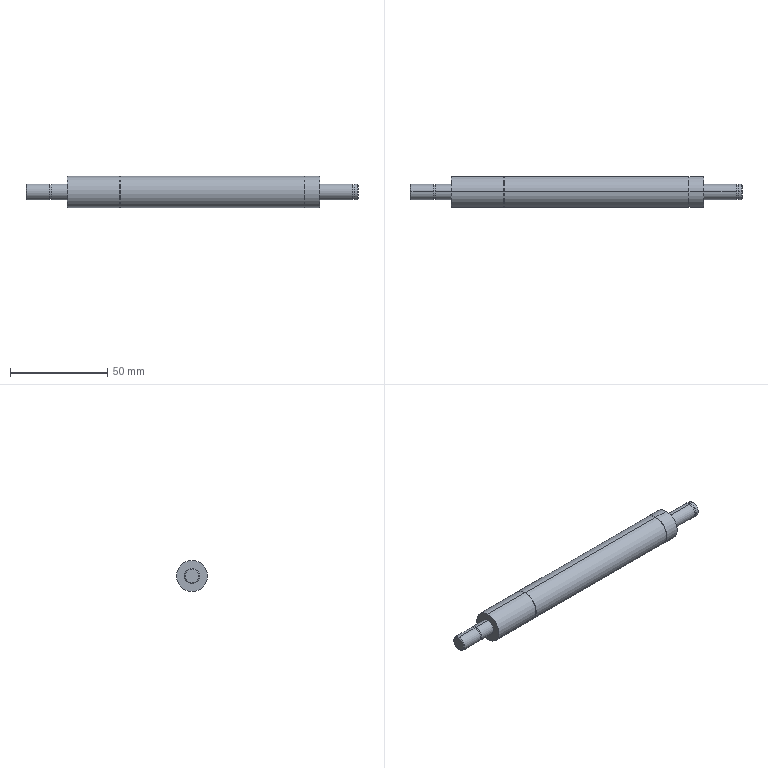Part | SolidWorks | features Chamfer 1, RevCut 1, Revolution 1 | 1 solid | 38 faces | box 171 x 16 x 16 mm | volume 28140 mm3 | cylinder 22 | plane 12 | cone 4 | commonest cylinder face diameters 8 x8 16 x6 7.6 x4 12.8 x4
STEP:
#1=CARTESIAN_POINT('',(171.,0.,-3.5));
#2=VERTEX_POINT('',#1);
#3=CARTESIAN_POINT('',(171.,0.,3.5));
#4=VERTEX_POINT('',#3);
#5=CARTESIAN_POINT('',(171.,0.,0.));
#6=DIRECTION('',(1.,0.,0.));
#7=DIRECTION('',(0.,0.,-1.));
#8=AXIS2_PLACEMENT_3D('',#5,#6,#7);
#9=CIRCLE('',#8,3.5);
#10=EDGE_CURVE('',#2,#4,#9,.T.);
#11=ORIENTED_EDGE('',*,*,#10,.F.);
#12=CARTESIAN_POINT('',(170.5,0.,-4.));
#13=VERTEX_POINT('',#12);
#14=CARTESIAN_POINT('',(170.5,0.,-4.));
#15=DIRECTION('',(-0.7071,0.,-0.7071));
#16=VECTOR('',#15,1000.);
#17=LINE('',#14,#16);
#18=EDGE_CURVE('',#2,#13,#17,.T.);
#19=ORIENTED_EDGE('',*,*,#18,.T.);
#20=CARTESIAN_POINT('',(170.5,0.,4.));
#21=VERTEX_POINT('',#20);
#22=CARTESIAN_POINT('',(170.5,0.,0.));
#23=DIRECTION('',(-1.,0.,0.));
#24=DIRECTION('',(0.,0.,-1.));
#25=AXIS2_PLACEMENT_3D('',#22,#23,#24);
#26=CIRCLE('',#25,4.);
#27=EDGE_CURVE('',#21,#13,#26,.T.);
#28=ORIENTED_EDGE('',*,*,#27,.F.);
#29=CARTESIAN_POINT('',(170.5,0.,4.));
#30=DIRECTION('',(-0.7071,0.,0.7071));
#31=VECTOR('',#30,1000.);
#32=LINE('',#29,#31);
#33=EDGE_CURVE('',#4,#21,#32,.T.);
#34=ORIENTED_EDGE('',*,*,#33,.F.);
#35=EDGE_LOOP('',(#11,#19,#28,#34));
#36=FACE_OUTER_BOUND('',#35,.T.);
#37=CARTESIAN_POINT('',(170.5,0.,0.));
#38=DIRECTION('',(-1.,0.,0.));
#39=DIRECTION('',(0.,0.,1.));
#40=AXIS2_PLACEMENT_3D('',#37,#38,#39);
#41=CONICAL_SURFACE('',#40,4.,0.7854);
#42=ADVANCED_FACE('',(#36),#41,.T.);
#43=CARTESIAN_POINT('',(0.,0.,3.5));
#44=VERTEX_POINT('',#43);
#45=CARTESIAN_POINT('',(0.,0.,-3.5));
#46=VERTEX_POINT('',#45);
#47=CARTESIAN_POINT('',(0.,0.,0.));
#48=DIRECTION('',(-1.,0.,0.));
#49=DIRECTION('',(0.,0.,1.));
#50=AXIS2_PLACEMENT_3D('',#47,#48,#49);
#51=CIRCLE('',#50,3.5);
#52=EDGE_CURVE('',#44,#46,#51,.T.);
#53=ORIENTED_EDGE('',*,*,#52,.F.);
#54=CARTESIAN_POINT('',(0.5,0.,4.));
#55=VERTEX_POINT('',#54);
#56=CARTESIAN_POINT('',(0.,0.,3.5));
#57=DIRECTION('',(0.7071,0.,0.7071));
#58=VECTOR('',#57,1000.);
#59=LINE('',#56,#58);
#60=EDGE_CURVE('',#44,#55,#59,.T.);
#61=ORIENTED_EDGE('',*,*,#60,.T.);
#62=CARTESIAN_POINT('',(0.5,0.,-4.));
#63=VERTEX_POINT('',#62);
#64=CARTESIAN_POINT('',(0.5,0.,0.));
#65=DIRECTION('',(1.,0.,0.));
#66=DIRECTION('',(0.,0.,1.));
#67=AXIS2_PLACEMENT_3D('',#64,#65,#66);
#68=CIRCLE('',#67,4.);
#69=EDGE_CURVE('',#63,#55,#68,.T.);
#70=ORIENTED_EDGE('',*,*,#69,.F.);
#71=CARTESIAN_POINT('',(0.,0.,-3.5));
#72=DIRECTION('',(0.7071,0.,-0.7071));
#73=VECTOR('',#72,1000.);
#74=LINE('',#71,#73);
#75=EDGE_CURVE('',#46,#63,#74,.T.);
#76=ORIENTED_EDGE('',*,*,#75,.F.);
#77=EDGE_LOOP('',(#53,#61,#70,#76));
#78=FACE_OUTER_BOUND('',#77,.T.);
#79=CARTESIAN_POINT('',(0.,0.,0.));
#80=DIRECTION('',(1.,0.,0.));
#81=DIRECTION('',(0.,0.,-1.));
#82=AXIS2_PLACEMENT_3D('',#79,#80,#81);
#83=CONICAL_SURFACE('',#82,3.5,0.7854);
#84=ADVANCED_FACE('',(#78),#83,.T.);
#85=CARTESIAN_POINT('',(12.,0.,4.));
#86=VERTEX_POINT('',#85);
#87=CARTESIAN_POINT('',(12.,0.,-4.));
#88=VERTEX_POINT('',#87);
#89=CARTESIAN_POINT('',(12.,0.,0.));
#90=DIRECTION('',(-1.,0.,0.));
#91=DIRECTION('',(0.,0.,1.));
#92=AXIS2_PLACEMENT_3D('',#89,#90,#91);
#93=CIRCLE('',#92,4.);
#94=EDGE_CURVE('',#86,#88,#93,.T.);
#95=ORIENTED_EDGE('',*,*,#94,.T.);
#96=CARTESIAN_POINT('',(-12.257,0.,-4.));
#97=DIRECTION('',(-1.,0.,0.));
#98=VECTOR('',#97,1000.);
#99=LINE('',#96,#98);
#100=EDGE_CURVE('',#88,#63,#99,.T.);
#101=ORIENTED_EDGE('',*,*,#100,.T.);
#102=ORIENTED_EDGE('',*,*,#69,.T.);
#103=CARTESIAN_POINT('',(-12.257,0.,4.));
#104=DIRECTION('',(-1.,0.,0.));
#105=VECTOR('',#104,1000.);
#106=LINE('',#103,#105);
#107=EDGE_CURVE('',#86,#55,#106,.T.);
#108=ORIENTED_EDGE('',*,*,#107,.F.);
#109=EDGE_LOOP('',(#95,#101,#102,#108));
#110=FACE_OUTER_BOUND('',#109,.T.);
#111=CARTESIAN_POINT('',(-12.257,0.,0.));
#112=DIRECTION('',(-1.,0.,0.));
#113=DIRECTION('',(0.,0.,1.));
#114=AXIS2_PLACEMENT_3D('',#111,#112,#113);
#115=CYLINDRICAL_SURFACE('',#114,4.);
#116=ADVANCED_FACE('',(#110),#115,.T.);
#117=CARTESIAN_POINT('',(12.9,0.,3.8));
#118=VERTEX_POINT('',#117);
#119=CARTESIAN_POINT('',(12.9,0.,-3.8));
#120=VERTEX_POINT('',#119);
#121=CARTESIAN_POINT('',(12.9,0.,0.));
#122=DIRECTION('',(-1.,0.,0.));
#123=DIRECTION('',(0.,0.,1.));
#124=AXIS2_PLACEMENT_3D('',#121,#122,#123);
#125=CIRCLE('',#124,3.8);
#126=EDGE_CURVE('',#118,#120,#125,.T.);
#127=ORIENTED_EDGE('',*,*,#126,.T.);
#128=CARTESIAN_POINT('',(12.,0.,-3.8));
#129=VERTEX_POINT('',#128);
#130=CARTESIAN_POINT('',(-6.355,0.,-3.8));
#131=DIRECTION('',(-1.,0.,0.));
#132=VECTOR('',#131,1000.);
#133=LINE('',#130,#132);
#134=EDGE_CURVE('',#120,#129,#133,.T.);
#135=ORIENTED_EDGE('',*,*,#134,.T.);
#136=CARTESIAN_POINT('',(12.,0.,3.8));
#137=VERTEX_POINT('',#136);
#138=CARTESIAN_POINT('',(12.,0.,0.));
#139=DIRECTION('',(-1.,0.,0.));
#140=DIRECTION('',(0.,0.,1.));
#141=AXIS2_PLACEMENT_3D('',#138,#139,#140);
#142=CIRCLE('',#141,3.8);
#143=EDGE_CURVE('',#137,#129,#142,.T.);
#144=ORIENTED_EDGE('',*,*,#143,.F.);
#145=CARTESIAN_POINT('',(-6.355,0.,3.8));
#146=DIRECTION('',(-1.,0.,0.));
#147=VECTOR('',#146,1000.);
#148=LINE('',#145,#147);
#149=EDGE_CURVE('',#118,#137,#148,.T.);
#150=ORIENTED_EDGE('',*,*,#149,.F.);
#151=EDGE_LOOP('',(#127,#135,#144,#150));
#152=FACE_OUTER_BOUND('',#151,.T.);
#153=CARTESIAN_POINT('',(-6.355,0.,0.));
#154=DIRECTION('',(-1.,0.,0.));
#155=DIRECTION('',(0.,0.,1.));
#156=AXIS2_PLACEMENT_3D('',#153,#154,#155);
#157=CYLINDRICAL_SURFACE('',#156,3.8);
#158=ADVANCED_FACE('',(#152),#157,.T.);
#159=ORIENTED_EDGE('',*,*,#27,.T.);
#160=CARTESIAN_POINT('',(169.,0.,-4.));
#161=VERTEX_POINT('',#160);
#162=CARTESIAN_POINT('',(-12.257,0.,-4.));
#163=DIRECTION('',(-1.,0.,0.));
#164=VECTOR('',#163,1000.);
#165=LINE('',#162,#164);
#166=EDGE_CURVE('',#13,#161,#165,.T.);
#167=ORIENTED_EDGE('',*,*,#166,.T.);
#168=CARTESIAN_POINT('',(169.,0.,4.));
#169=VERTEX_POINT('',#168);
#170=CARTESIAN_POINT('',(169.,0.,0.));
#171=DIRECTION('',(-1.,0.,0.));
#172=DIRECTION('',(0.,0.,1.));
#173=AXIS2_PLACEMENT_3D('',#170,#171,#172);
#174=CIRCLE('',#173,4.);
#175=EDGE_CURVE('',#169,#161,#174,.T.);
#176=ORIENTED_EDGE('',*,*,#175,.F.);
#177=CARTESIAN_POINT('',(-12.257,0.,4.));
#178=DIRECTION('',(-1.,0.,0.));
#179=VECTOR('',#178,1000.);
#180=LINE('',#177,#179);
#181=EDGE_CURVE('',#21,#169,#180,.T.);
#182=ORIENTED_EDGE('',*,*,#181,.F.);
#183=EDGE_LOOP('',(#159,#167,#176,#182));
#184=FACE_OUTER_BOUND('',#183,.T.);
#185=CARTESIAN_POINT('',(-12.257,0.,0.));
#186=DIRECTION('',(-1.,0.,0.));
#187=DIRECTION('',(0.,0.,1.));
#188=AXIS2_PLACEMENT_3D('',#185,#186,#187);
#189=CYLINDRICAL_SURFACE('',#188,4.);
#190=ADVANCED_FACE('',(#184),#189,.T.);
#191=CARTESIAN_POINT('',(169.,0.,3.8));
#192=VERTEX_POINT('',#191);
#193=CARTESIAN_POINT('',(169.,0.,-3.8));
#194=VERTEX_POINT('',#193);
#195=CARTESIAN_POINT('',(169.,0.,0.));
#196=DIRECTION('',(-1.,0.,0.));
#197=DIRECTION('',(0.,0.,1.));
#198=AXIS2_PLACEMENT_3D('',#195,#196,#197);
#199=CIRCLE('',#198,3.8);
#200=EDGE_CURVE('',#192,#194,#199,.T.);
#201=ORIENTED_EDGE('',*,*,#200,.T.);
#202=CARTESIAN_POINT('',(168.1,0.,-3.8));
#203=VERTEX_POINT('',#202);
#204=CARTESIAN_POINT('',(-6.355,0.,-3.8));
#205=DIRECTION('',(-1.,0.,0.));
#206=VECTOR('',#205,1000.);
#207=LINE('',#204,#206);
#208=EDGE_CURVE('',#194,#203,#207,.T.);
#209=ORIENTED_EDGE('',*,*,#208,.T.);
#210=CARTESIAN_POINT('',(168.1,0.,3.8));
#211=VERTEX_POINT('',#210);
#212=CARTESIAN_POINT('',(168.1,0.,0.));
#213=DIRECTION('',(-1.,0.,0.));
#214=DIRECTION('',(0.,0.,1.));
#215=AXIS2_PLACEMENT_3D('',#212,#213,#214);
#216=CIRCLE('',#215,3.8);
#217=EDGE_CURVE('',#211,#203,#216,.T.);
#218=ORIENTED_EDGE('',*,*,#217,.F.);
#219=CARTESIAN_POINT('',(-6.355,0.,3.8));
#220=DIRECTION('',(-1.,0.,0.));
#221=VECTOR('',#220,1000.);
#222=LINE('',#219,#221);
#223=EDGE_CURVE('',#192,#211,#222,.T.);
#224=ORIENTED_EDGE('',*,*,#223,.F.);
#225=EDGE_LOOP('',(#201,#209,#218,#224));
#226=FACE_OUTER_BOUND('',#225,.T.);
#227=CARTESIAN_POINT('',(-6.355,0.,0.));
#228=DIRECTION('',(-1.,0.,0.));
#229=DIRECTION('',(0.,0.,1.));
#230=AXIS2_PLACEMENT_3D('',#227,#228,#229);
#231=CYLINDRICAL_SURFACE('',#230,3.8);
#232=ADVANCED_FACE('',(#226),#231,.T.);
#233=CARTESIAN_POINT('',(151.2,0.,8.));
#234=VERTEX_POINT('',#233);
#235=CARTESIAN_POINT('',(151.2,0.,-8.));
#236=VERTEX_POINT('',#235);
#237=CARTESIAN_POINT('',(151.2,0.,0.));
#238=DIRECTION('',(-1.,0.,0.));
#239=DIRECTION('',(0.,0.,1.));
#240=AXIS2_PLACEMENT_3D('',#237,#238,#239);
#241=CIRCLE('',#240,8.);
#242=EDGE_CURVE('',#234,#236,#241,.T.);
#243=ORIENTED_EDGE('',*,*,#242,.T.);
#244=CARTESIAN_POINT('',(143.7,0.,-8.));
#245=VERTEX_POINT('',#244);
#246=CARTESIAN_POINT('',(-12.257,0.,-8.));
#247=DIRECTION('',(-1.,0.,0.));
#248=VECTOR('',#247,1000.);
#249=LINE('',#246,#248);
#250=EDGE_CURVE('',#236,#245,#249,.T.);
#251=ORIENTED_EDGE('',*,*,#250,.T.);
#252=CARTESIAN_POINT('',(143.7,0.,8.));
#253=VERTEX_POINT('',#252);
#254=CARTESIAN_POINT('',(143.7,0.,0.));
#255=DIRECTION('',(-1.,0.,0.));
#256=DIRECTION('',(0.,0.,1.));
#257=AXIS2_PLACEMENT_3D('',#254,#255,#256);
#258=CIRCLE('',#257,8.);
#259=EDGE_CURVE('',#253,#245,#258,.T.);
#260=ORIENTED_EDGE('',*,*,#259,.F.);
#261=CARTESIAN_POINT('',(-12.257,0.,8.));
#262=DIRECTION('',(-1.,0.,0.));
#263=VECTOR('',#262,1000.);
#264=LINE('',#261,#263);
#265=EDGE_CURVE('',#234,#253,#264,.T.);
#266=ORIENTED_EDGE('',*,*,#265,.F.);
#267=EDGE_LOOP('',(#243,#251,#260,#266));
#268=FACE_OUTER_BOUND('',#267,.T.);
#269=CARTESIAN_POINT('',(-12.257,0.,0.));
#270=DIRECTION('',(-1.,0.,0.));
#271=DIRECTION('',(0.,0.,1.));
#272=AXIS2_PLACEMENT_3D('',#269,#270,#271);
#273=CYLINDRICAL_SURFACE('',#272,8.);
#274=ADVANCED_FACE('',(#268),#273,.T.);
#275=CARTESIAN_POINT('',(143.7,0.,6.4));
#276=VERTEX_POINT('',#275);
#277=CARTESIAN_POINT('',(143.7,0.,-6.4));
#278=VERTEX_POINT('',#277);
#279=CARTESIAN_POINT('',(143.7,0.,0.));
#280=DIRECTION('',(-1.,0.,0.));
#281=DIRECTION('',(0.,0.,1.));
#282=AXIS2_PLACEMENT_3D('',#279,#280,#281);
#283=CIRCLE('',#282,6.4);
#284=EDGE_CURVE('',#276,#278,#283,.T.);
#285=ORIENTED_EDGE('',*,*,#284,.T.);
#286=CARTESIAN_POINT('',(143.5,0.,-6.4));
#287=VERTEX_POINT('',#286);
#288=CARTESIAN_POINT('',(-6.355,0.,-6.4));
#289=DIRECTION('',(-1.,0.,0.));
#290=VECTOR('',#289,1000.);
#291=LINE('',#288,#290);
#292=EDGE_CURVE('',#278,#287,#291,.T.);
#293=ORIENTED_EDGE('',*,*,#292,.T.);
#294=CARTESIAN_POINT('',(143.5,0.,6.4));
#295=VERTEX_POINT('',#294);
#296=CARTESIAN_POINT('',(143.5,0.,0.));
#297=DIRECTION('',(-1.,0.,0.));
#298=DIRECTION('',(0.,0.,1.));
#299=AXIS2_PLACEMENT_3D('',#296,#297,#298);
#300=CIRCLE('',#299,6.4);
#301=EDGE_CURVE('',#295,#287,#300,.T.);
#302=ORIENTED_EDGE('',*,*,#301,.F.);
#303=CARTESIAN_POINT('',(-6.355,0.,6.4));
#304=DIRECTION('',(-1.,0.,0.));
#305=VECTOR('',#304,1000.);
#306=LINE('',#303,#305);
#307=EDGE_CURVE('',#276,#295,#306,.T.);
#308=ORIENTED_EDGE('',*,*,#307,.F.);
#309=EDGE_LOOP('',(#285,#293,#302,#308));
#310=FACE_OUTER_BOUND('',#309,.T.);
#311=CARTESIAN_POINT('',(-6.355,0.,0.));
#312=DIRECTION('',(-1.,0.,0.));
#313=DIRECTION('',(0.,0.,1.));
#314=AXIS2_PLACEMENT_3D('',#311,#312,#313);
#315=CYLINDRICAL_SURFACE('',#314,6.4);
#316=ADVANCED_FACE('',(#310),#315,.T.);
#317=CARTESIAN_POINT('',(48.5,0.,6.4));
#318=VERTEX_POINT('',#317);
#319=CARTESIAN_POINT('',(48.5,0.,-6.4));
#320=VERTEX_POINT('',#319);
#321=CARTESIAN_POINT('',(48.5,0.,0.));
#322=DIRECTION('',(-1.,0.,0.));
#323=DIRECTION('',(0.,0.,1.));
#324=AXIS2_PLACEMENT_3D('',#321,#322,#323);
#325=CIRCLE('',#324,6.4);
#326=EDGE_CURVE('',#318,#320,#325,.T.);
#327=ORIENTED_EDGE('',*,*,#326,.T.);
#328=CARTESIAN_POINT('',(48.3,0.,-6.4));
#329=VERTEX_POINT('',#328);
#330=CARTESIAN_POINT('',(-6.355,0.,-6.4));
#331=DIRECTION('',(-1.,0.,0.));
#332=VECTOR('',#331,1000.);
#333=LINE('',#330,#332);
#334=EDGE_CURVE('',#320,#329,#333,.T.);
#335=ORIENTED_EDGE('',*,*,#334,.T.);
#336=CARTESIAN_POINT('',(48.3,0.,6.4));
#337=VERTEX_POINT('',#336);
#338=CARTESIAN_POINT('',(48.3,0.,0.));
#339=DIRECTION('',(-1.,0.,0.));
#340=DIRECTION('',(0.,0.,1.));
#341=AXIS2_PLACEMENT_3D('',#338,#339,#340);
#342=CIRCLE('',#341,6.4);
#343=EDGE_CURVE('',#337,#329,#342,.T.);
#344=ORIENTED_EDGE('',*,*,#343,.F.);
#345=CARTESIAN_POINT('',(-6.355,0.,6.4));
#346=DIRECTION('',(-1.,0.,0.));
#347=VECTOR('',#346,1000.);
#348=LINE('',#345,#347);
#349=EDGE_CURVE('',#318,#337,#348,.T.);
#350=ORIENTED_EDGE('',*,*,#349,.F.);
#351=EDGE_LOOP('',(#327,#335,#344,#350));
#352=FACE_OUTER_BOUND('',#351,.T.);
#353=CARTESIAN_POINT('',(-6.355,0.,0.));
#354=DIRECTION('',(-1.,0.,0.));
#355=DIRECTION('',(0.,0.,1.));
#356=AXIS2_PLACEMENT_3D('',#353,#354,#355);
#357=CYLINDRICAL_SURFACE('',#356,6.4);
#358=ADVANCED_FACE('',(#352),#357,.T.);
#359=CARTESIAN_POINT('',(21.3,0.,4.));
#360=VERTEX_POINT('',#359);
#361=CARTESIAN_POINT('',(21.3,0.,-4.));
#362=VERTEX_POINT('',#361);
#363=CARTESIAN_POINT('',(21.3,0.,0.));
#364=DIRECTION('',(-1.,0.,0.));
#365=DIRECTION('',(0.,0.,1.));
#366=AXIS2_PLACEMENT_3D('',#363,#364,#365);
#367=CIRCLE('',#366,4.);
#368=EDGE_CURVE('',#360,#362,#367,.T.);
#369=ORIENTED_EDGE('',*,*,#368,.T.);
#370=CARTESIAN_POINT('',(12.9,0.,-4.));
#371=VERTEX_POINT('',#370);
#372=CARTESIAN_POINT('',(-12.257,0.,-4.));
#373=DIRECTION('',(-1.,0.,0.));
#374=VECTOR('',#373,1000.);
#375=LINE('',#372,#374);
#376=EDGE_CURVE('',#362,#371,#375,.T.);
#377=ORIENTED_EDGE('',*,*,#376,.T.);
#378=CARTESIAN_POINT('',(12.9,0.,4.));
#379=VERTEX_POINT('',#378);
#380=CARTESIAN_POINT('',(12.9,0.,0.));
#381=DIRECTION('',(-1.,0.,0.));
#382=DIRECTION('',(0.,0.,1.));
#383=AXIS2_PLACEMENT_3D('',#380,#381,#382);
#384=CIRCLE('',#383,4.);
#385=EDGE_CURVE('',#379,#371,#384,.T.);
#386=ORIENTED_EDGE('',*,*,#385,.F.);
#387=CARTESIAN_POINT('',(-12.257,0.,4.));
#388=DIRECTION('',(-1.,0.,0.));
#389=VECTOR('',#388,1000.);
#390=LINE('',#387,#389);
#391=EDGE_CURVE('',#360,#379,#390,.T.);
#392=ORIENTED_EDGE('',*,*,#391,.F.);
#393=EDGE_LOOP('',(#369,#377,#386,#392));
#394=FACE_OUTER_BOUND('',#393,.T.);
#395=CARTESIAN_POINT('',(-12.257,0.,0.));
#396=DIRECTION('',(-1.,0.,0.));
#397=DIRECTION('',(0.,0.,1.));
#398=AXIS2_PLACEMENT_3D('',#395,#396,#397);
#399=CYLINDRICAL_SURFACE('',#398,4.);
#400=ADVANCED_FACE('',(#394),#399,.T.);
#401=CARTESIAN_POINT('',(48.3,0.,8.));
#402=VERTEX_POINT('',#401);
#403=CARTESIAN_POINT('',(48.3,0.,-8.));
#404=VERTEX_POINT('',#403);
#405=CARTESIAN_POINT('',(48.3,0.,0.));
#406=DIRECTION('',(-1.,0.,0.));
#407=DIRECTION('',(0.,0.,1.));
#408=AXIS2_PLACEMENT_3D('',#405,#406,#407);
#409=CIRCLE('',#408,8.);
#410=EDGE_CURVE('',#402,#404,#409,.T.);
#411=ORIENTED_EDGE('',*,*,#410,.T.);
#412=CARTESIAN_POINT('',(21.3,0.,-8.));
#413=VERTEX_POINT('',#412);
#414=CARTESIAN_POINT('',(-12.257,0.,-8.));
#415=DIRECTION('',(-1.,0.,0.));
#416=VECTOR('',#415,1000.);
#417=LINE('',#414,#416);
#418=EDGE_CURVE('',#404,#413,#417,.T.);
#419=ORIENTED_EDGE('',*,*,#418,.T.);
#420=CARTESIAN_POINT('',(21.3,0.,8.));
#421=VERTEX_POINT('',#420);
#422=CARTESIAN_POINT('',(21.3,0.,0.));
#423=DIRECTION('',(-1.,0.,0.));
#424=DIRECTION('',(0.,0.,1.));
#425=AXIS2_PLACEMENT_3D('',#422,#423,#424);
#426=CIRCLE('',#425,8.);
#427=EDGE_CURVE('',#421,#413,#426,.T.);
#428=ORIENTED_EDGE('',*,*,#427,.F.);
#429=CARTESIAN_POINT('',(-12.257,0.,8.));
#430=DIRECTION('',(-1.,0.,0.));
#431=VECTOR('',#430,1000.);
#432=LINE('',#429,#431);
#433=EDGE_CURVE('',#402,#421,#432,.T.);
#434=ORIENTED_EDGE('',*,*,#433,.F.);
#435=EDGE_LOOP('',(#411,#419,#428,#434));
#436=FACE_OUTER_BOUND('',#435,.T.);
#437=CARTESIAN_POINT('',(-12.257,0.,0.));
#438=DIRECTION('',(-1.,0.,0.));
#439=DIRECTION('',(0.,0.,1.));
#440=AXIS2_PLACEMENT_3D('',#437,#438,#439);
#441=CYLINDRICAL_SURFACE('',#440,8.);
#442=ADVANCED_FACE('',(#436),#441,.T.);
#443=CARTESIAN_POINT('',(143.5,0.,8.));
#444=VERTEX_POINT('',#443);
#445=CARTESIAN_POINT('',(143.5,0.,-8.));
#446=VERTEX_POINT('',#445);
#447=CARTESIAN_POINT('',(143.5,0.,0.));
#448=DIRECTION('',(-1.,0.,0.));
#449=DIRECTION('',(0.,0.,1.));
#450=AXIS2_PLACEMENT_3D('',#447,#448,#449);
#451=CIRCLE('',#450,8.);
#452=EDGE_CURVE('',#444,#446,#451,.T.);
#453=ORIENTED_EDGE('',*,*,#452,.T.);
#454=CARTESIAN_POINT('',(48.5,0.,-8.));
#455=VERTEX_POINT('',#454);
#456=CARTESIAN_POINT('',(-12.257,0.,-8.));
#457=DIRECTION('',(-1.,0.,0.));
#458=VECTOR('',#457,1000.);
#459=LINE('',#456,#458);
#460=EDGE_CURVE('',#446,#455,#459,.T.);
#461=ORIENTED_EDGE('',*,*,#460,.T.);
#462=CARTESIAN_POINT('',(48.5,0.,8.));
#463=VERTEX_POINT('',#462);
#464=CARTESIAN_POINT('',(48.5,0.,0.));
#465=DIRECTION('',(-1.,0.,0.));
#466=DIRECTION('',(0.,0.,1.));
#467=AXIS2_PLACEMENT_3D('',#464,#465,#466);
#468=CIRCLE('',#467,8.);
#469=EDGE_CURVE('',#463,#455,#468,.T.);
#470=ORIENTED_EDGE('',*,*,#469,.F.);
#471=CARTESIAN_POINT('',(-12.257,0.,8.));
#472=DIRECTION('',(-1.,0.,0.));
#473=VECTOR('',#472,1000.);
#474=LINE('',#471,#473);
#475=EDGE_CURVE('',#444,#463,#474,.T.);
#476=ORIENTED_EDGE('',*,*,#475,.F.);
#477=EDGE_LOOP('',(#453,#461,#470,#476));
#478=FACE_OUTER_BOUND('',#477,.T.);
#479=CARTESIAN_POINT('',(-12.257,0.,0.));
#480=DIRECTION('',(-1.,0.,0.));
#481=DIRECTION('',(0.,0.,1.));
#482=AXIS2_PLACEMENT_3D('',#479,#480,#481);
#483=CYLINDRICAL_SURFACE('',#482,8.);
#484=ADVANCED_FACE('',(#478),#483,.T.);
#485=CARTESIAN_POINT('',(168.1,0.,4.));
#486=VERTEX_POINT('',#485);
#487=CARTESIAN_POINT('',(168.1,0.,-4.));
#488=VERTEX_POINT('',#487);
#489=CARTESIAN_POINT('',(168.1,0.,0.));
#490=DIRECTION('',(-1.,0.,0.));
#491=DIRECTION('',(0.,0.,1.));
#492=AXIS2_PLACEMENT_3D('',#489,#490,#491);
#493=CIRCLE('',#492,4.);
#494=EDGE_CURVE('',#486,#488,#493,.T.);
#495=ORIENTED_EDGE('',*,*,#494,.T.);
#496=CARTESIAN_POINT('',(151.2,0.,-4.));
#497=VERTEX_POINT('',#496);
#498=CARTESIAN_POINT('',(-12.257,0.,-4.));
#499=DIRECTION('',(-1.,0.,0.));
#500=VECTOR('',#499,1000.);
#501=LINE('',#498,#500);
#502=EDGE_CURVE('',#488,#497,#501,.T.);
#503=ORIENTED_EDGE('',*,*,#502,.T.);
#504=CARTESIAN_POINT('',(151.2,0.,4.));
#505=VERTEX_POINT('',#504);
#506=CARTESIAN_POINT('',(151.2,0.,0.));
#507=DIRECTION('',(-1.,0.,0.));
#508=DIRECTION('',(0.,0.,1.));
#509=AXIS2_PLACEMENT_3D('',#506,#507,#508);
#510=CIRCLE('',#509,4.);
#511=EDGE_CURVE('',#505,#497,#510,.T.);
#512=ORIENTED_EDGE('',*,*,#511,.F.);
#513=CARTESIAN_POINT('',(-12.257,0.,4.));
#514=DIRECTION('',(-1.,0.,0.));
#515=VECTOR('',#514,1000.);
#516=LINE('',#513,#515);
#517=EDGE_CURVE('',#486,#505,#516,.T.);
#518=ORIENTED_EDGE('',*,*,#517,.F.);
#519=EDGE_LOOP('',(#495,#503,#512,#518));
#520=FACE_OUTER_BOUND('',#519,.T.);
#521=CARTESIAN_POINT('',(-12.257,0.,0.));
#522=DIRECTION('',(-1.,0.,0.));
#523=DIRECTION('',(0.,0.,1.));
#524=AXIS2_PLACEMENT_3D('',#521,#522,#523);
#525=CYLINDRICAL_SURFACE('',#524,4.);
#526=ADVANCED_FACE('',(#520),#525,.T.);
#527=ORIENTED_EDGE('',*,*,#502,.F.);
#528=CARTESIAN_POINT('',(168.1,0.,0.));
#529=DIRECTION('',(-1.,0.,0.));
#530=DIRECTION('',(0.,0.,1.));
#531=AXIS2_PLACEMENT_3D('',#528,#529,#530);
#532=CIRCLE('',#531,4.);
#533=EDGE_CURVE('',#488,#486,#532,.T.);
#534=ORIENTED_EDGE('',*,*,#533,.T.);
#535=ORIENTED_EDGE('',*,*,#517,.T.);
#536=CARTESIAN_POINT('',(151.2,0.,0.));
#537=DIRECTION('',(-1.,0.,0.));
#538=DIRECTION('',(0.,0.,1.));
#539=AXIS2_PLACEMENT_3D('',#536,#537,#538);
#540=CIRCLE('',#539,4.);
#541=EDGE_CURVE('',#497,#505,#540,.T.);
#542=ORIENTED_EDGE('',*,*,#541,.F.);
#543=EDGE_LOOP('',(#527,#534,#535,#542));
#544=FACE_OUTER_BOUND('',#543,.T.);
#545=CARTESIAN_POINT('',(-12.257,0.,0.));
#546=DIRECTION('',(-1.,0.,0.));
#547=DIRECTION('',(0.,0.,1.));
#548=AXIS2_PLACEMENT_3D('',#545,#546,#547);
#549=CYLINDRICAL_SURFACE('',#548,4.);
#550=ADVANCED_FACE('',(#544),#549,.T.);
#551=ORIENTED_EDGE('',*,*,#460,.F.);
#552=CARTESIAN_POINT('',(143.5,0.,0.));
#553=DIRECTION('',(-1.,0.,0.));
#554=DIRECTION('',(0.,0.,1.));
#555=AXIS2_PLACEMENT_3D('',#552,#553,#554);
#556=CIRCLE('',#555,8.);
#557=EDGE_CURVE('',#446,#444,#556,.T.);
#558=ORIENTED_EDGE('',*,*,#557,.T.);
#559=ORIENTED_EDGE('',*,*,#475,.T.);
#560=CARTESIAN_POINT('',(48.5,0.,0.));
#561=DIRECTION('',(-1.,0.,0.));
#562=DIRECTION('',(0.,0.,1.));
#563=AXIS2_PLACEMENT_3D('',#560,#561,#562);
#564=CIRCLE('',#563,8.);
#565=EDGE_CURVE('',#455,#463,#564,.T.);
#566=ORIENTED_EDGE('',*,*,#565,.F.);
#567=EDGE_LOOP('',(#551,#558,#559,#566));
#568=FACE_OUTER_BOUND('',#567,.T.);
#569=CARTESIAN_POINT('',(-12.257,0.,0.));
#570=DIRECTION('',(-1.,0.,0.));
#571=DIRECTION('',(0.,0.,1.));
#572=AXIS2_PLACEMENT_3D('',#569,#570,#571);
#573=CYLINDRICAL_SURFACE('',#572,8.);
#574=ADVANCED_FACE('',(#568),#573,.T.);
#575=ORIENTED_EDGE('',*,*,#418,.F.);
#576=CARTESIAN_POINT('',(48.3,0.,0.));
#577=DIRECTION('',(-1.,0.,0.));
#578=DIRECTION('',(0.,0.,1.));
#579=AXIS2_PLACEMENT_3D('',#576,#577,#578);
#580=CIRCLE('',#579,8.);
#581=EDGE_CURVE('',#404,#402,#580,.T.);
#582=ORIENTED_EDGE('',*,*,#581,.T.);
#583=ORIENTED_EDGE('',*,*,#433,.T.);
#584=CARTESIAN_POINT('',(21.3,0.,0.));
#585=DIRECTION('',(-1.,0.,0.));
#586=DIRECTION('',(0.,0.,1.));
#587=AXIS2_PLACEMENT_3D('',#584,#585,#586);
#588=CIRCLE('',#587,8.);
#589=EDGE_CURVE('',#413,#421,#588,.T.);
#590=ORIENTED_EDGE('',*,*,#589,.F.);
#591=EDGE_LOOP('',(#575,#582,#583,#590));
#592=FACE_OUTER_BOUND('',#591,.T.);
#593=CARTESIAN_POINT('',(-12.257,0.,0.));
#594=DIRECTION('',(-1.,0.,0.));
#595=DIRECTION('',(0.,0.,1.));
#596=AXIS2_PLACEMENT_3D('',#593,#594,#595);
#597=CYLINDRICAL_SURFACE('',#596,8.);
#598=ADVANCED_FACE('',(#592),#597,.T.);
#599=ORIENTED_EDGE('',*,*,#376,.F.);
#600=CARTESIAN_POINT('',(21.3,0.,0.));
#601=DIRECTION('',(-1.,0.,0.));
#602=DIRECTION('',(0.,0.,1.));
#603=AXIS2_PLACEMENT_3D('',#600,#601,#602);
#604=CIRCLE('',#603,4.);
#605=EDGE_CURVE('',#362,#360,#604,.T.);
#606=ORIENTED_EDGE('',*,*,#605,.T.);
#607=ORIENTED_EDGE('',*,*,#391,.T.);
#608=CARTESIAN_POINT('',(12.9,0.,0.));
#609=DIRECTION('',(-1.,0.,0.));
#610=DIRECTION('',(0.,0.,1.));
#611=AXIS2_PLACEMENT_3D('',#608,#609,#610);
#612=CIRCLE('',#611,4.);
#613=EDGE_CURVE('',#371,#379,#612,.T.);
#614=ORIENTED_EDGE('',*,*,#613,.F.);
#615=EDGE_LOOP('',(#599,#606,#607,#614));
#616=FACE_OUTER_BOUND('',#615,.T.);
#617=CARTESIAN_POINT('',(-12.257,0.,0.));
#618=DIRECTION('',(-1.,0.,0.));
#619=DIRECTION('',(0.,0.,1.));
#620=AXIS2_PLACEMENT_3D('',#617,#618,#619);
#621=CYLINDRICAL_SURFACE('',#620,4.);
#622=ADVANCED_FACE('',(#616),#621,.T.);
#623=ORIENTED_EDGE('',*,*,#427,.T.);
#624=ORIENTED_EDGE('',*,*,#589,.T.);
#625=EDGE_LOOP('',(#623,#624));
#626=FACE_OUTER_BOUND('',#625,.T.);
#627=ORIENTED_EDGE('',*,*,#368,.F.);
#628=ORIENTED_EDGE('',*,*,#605,.F.);
#629=EDGE_LOOP('',(#627,#628));
#630=FACE_BOUND('',#629,.T.);
#631=CARTESIAN_POINT('',(21.3,0.,-4.));
#632=DIRECTION('',(-1.,0.,0.));
#633=DIRECTION('',(0.,0.,1.));
#634=AXIS2_PLACEMENT_3D('',#631,#632,#633);
#635=PLANE('',#634);
#636=ADVANCED_FACE('',(#626,#630),#635,.T.);
#637=ORIENTED_EDGE('',*,*,#410,.F.);
#638=ORIENTED_EDGE('',*,*,#581,.F.);
#639=EDGE_LOOP('',(#637,#638));
#640=FACE_OUTER_BOUND('',#639,.T.);
#641=ORIENTED_EDGE('',*,*,#343,.T.);
#642=CARTESIAN_POINT('',(48.3,0.,0.));
#643=DIRECTION('',(-1.,0.,0.));
#644=DIRECTION('',(0.,0.,1.));
#645=AXIS2_PLACEMENT_3D('',#642,#643,#644);
#646=CIRCLE('',#645,6.4);
#647=EDGE_CURVE('',#329,#337,#646,.T.);
#648=ORIENTED_EDGE('',*,*,#647,.T.);
#649=EDGE_LOOP('',(#641,#648));
#650=FACE_BOUND('',#649,.T.);
#651=CARTESIAN_POINT('',(48.3,0.,-8.));
#652=DIRECTION('',(-1.,0.,0.));
#653=DIRECTION('',(0.,0.,1.));
#654=AXIS2_PLACEMENT_3D('',#651,#652,#653);
#655=PLANE('',#654);
#656=ADVANCED_FACE('',(#640,#650),#655,.F.);
#657=ORIENTED_EDGE('',*,*,#334,.F.);
#658=CARTESIAN_POINT('',(48.5,0.,0.));
#659=DIRECTION('',(-1.,0.,0.));
#660=DIRECTION('',(0.,0.,1.));
#661=AXIS2_PLACEMENT_3D('',#658,#659,#660);
#662=CIRCLE('',#661,6.4);
#663=EDGE_CURVE('',#320,#318,#662,.T.);
#664=ORIENTED_EDGE('',*,*,#663,.T.);
#665=ORIENTED_EDGE('',*,*,#349,.T.);
#666=ORIENTED_EDGE('',*,*,#647,.F.);
#667=EDGE_LOOP('',(#657,#664,#665,#666));
#668=FACE_OUTER_BOUND('',#667,.T.);
#669=CARTESIAN_POINT('',(-6.355,0.,0.));
#670=DIRECTION('',(-1.,0.,0.));
#671=DIRECTION('',(0.,0.,1.));
#672=AXIS2_PLACEMENT_3D('',#669,#670,#671);
#673=CYLINDRICAL_SURFACE('',#672,6.4);
#674=ADVANCED_FACE('',(#668),#673,.T.);
#675=ORIENTED_EDGE('',*,*,#326,.F.);
#676=ORIENTED_EDGE('',*,*,#663,.F.);
#677=EDGE_LOOP('',(#675,#676));
#678=FACE_BOUND('',#677,.T.);
#679=ORIENTED_EDGE('',*,*,#469,.T.);
#680=ORIENTED_EDGE('',*,*,#565,.T.);
#681=EDGE_LOOP('',(#679,#680));
#682=FACE_OUTER_BOUND('',#681,.T.);
#683=CARTESIAN_POINT('',(48.5,0.,-8.));
#684=DIRECTION('',(1.,0.,0.));
#685=DIRECTION('',(0.,0.,-1.));
#686=AXIS2_PLACEMENT_3D('',#683,#684,#685);
#687=PLANE('',#686);
#688=ADVANCED_FACE('',(#678,#682),#687,.F.);
#689=ORIENTED_EDGE('',*,*,#452,.F.);
#690=ORIENTED_EDGE('',*,*,#557,.F.);
#691=EDGE_LOOP('',(#689,#690));
#692=FACE_OUTER_BOUND('',#691,.T.);
#693=ORIENTED_EDGE('',*,*,#301,.T.);
#694=CARTESIAN_POINT('',(143.5,0.,0.));
#695=DIRECTION('',(-1.,0.,0.));
#696=DIRECTION('',(0.,0.,1.));
#697=AXIS2_PLACEMENT_3D('',#694,#695,#696);
#698=CIRCLE('',#697,6.4);
#699=EDGE_CURVE('',#287,#295,#698,.T.);
#700=ORIENTED_EDGE('',*,*,#699,.T.);
#701=EDGE_LOOP('',(#693,#700));
#702=FACE_BOUND('',#701,.T.);
#703=CARTESIAN_POINT('',(143.5,0.,-8.));
#704=DIRECTION('',(-1.,0.,0.));
#705=DIRECTION('',(0.,0.,1.));
#706=AXIS2_PLACEMENT_3D('',#703,#704,#705);
#707=PLANE('',#706);
#708=ADVANCED_FACE('',(#692,#702),#707,.F.);
#709=ORIENTED_EDGE('',*,*,#292,.F.);
#710=CARTESIAN_POINT('',(143.7,0.,0.));
#711=DIRECTION('',(-1.,0.,0.));
#712=DIRECTION('',(0.,0.,1.));
#713=AXIS2_PLACEMENT_3D('',#710,#711,#712);
#714=CIRCLE('',#713,6.4);
#715=EDGE_CURVE('',#278,#276,#714,.T.);
#716=ORIENTED_EDGE('',*,*,#715,.T.);
#717=ORIENTED_EDGE('',*,*,#307,.T.);
#718=ORIENTED_EDGE('',*,*,#699,.F.);
#719=EDGE_LOOP('',(#709,#716,#717,#718));
#720=FACE_OUTER_BOUND('',#719,.T.);
#721=CARTESIAN_POINT('',(-6.355,0.,0.));
#722=DIRECTION('',(-1.,0.,0.));
#723=DIRECTION('',(0.,0.,1.));
#724=AXIS2_PLACEMENT_3D('',#721,#722,#723);
#725=CYLINDRICAL_SURFACE('',#724,6.4);
#726=ADVANCED_FACE('',(#720),#725,.T.);
#727=ORIENTED_EDGE('',*,*,#284,.F.);
#728=ORIENTED_EDGE('',*,*,#715,.F.);
#729=EDGE_LOOP('',(#727,#728));
#730=FACE_BOUND('',#729,.T.);
#731=ORIENTED_EDGE('',*,*,#259,.T.);
#732=CARTESIAN_POINT('',(143.7,0.,0.));
#733=DIRECTION('',(-1.,0.,0.));
#734=DIRECTION('',(0.,0.,1.));
#735=AXIS2_PLACEMENT_3D('',#732,#733,#734);
#736=CIRCLE('',#735,8.);
#737=EDGE_CURVE('',#245,#253,#736,.T.);
#738=ORIENTED_EDGE('',*,*,#737,.T.);
#739=EDGE_LOOP('',(#731,#738));
#740=FACE_OUTER_BOUND('',#739,.T.);
#741=CARTESIAN_POINT('',(143.7,0.,-8.));
#742=DIRECTION('',(1.,0.,0.));
#743=DIRECTION('',(0.,0.,-1.));
#744=AXIS2_PLACEMENT_3D('',#741,#742,#743);
#745=PLANE('',#744);
#746=ADVANCED_FACE('',(#730,#740),#745,.F.);
#747=ORIENTED_EDGE('',*,*,#511,.T.);
#748=ORIENTED_EDGE('',*,*,#541,.T.);
#749=EDGE_LOOP('',(#747,#748));
#750=FACE_BOUND('',#749,.T.);
#751=ORIENTED_EDGE('',*,*,#242,.F.);
#752=CARTESIAN_POINT('',(151.2,0.,0.));
#753=DIRECTION('',(-1.,0.,0.));
#754=DIRECTION('',(0.,0.,1.));
#755=AXIS2_PLACEMENT_3D('',#752,#753,#754);
#756=CIRCLE('',#755,8.);
#757=EDGE_CURVE('',#236,#234,#756,.T.);
#758=ORIENTED_EDGE('',*,*,#757,.F.);
#759=EDGE_LOOP('',(#751,#758));
#760=FACE_OUTER_BOUND('',#759,.T.);
#761=CARTESIAN_POINT('',(151.2,0.,-8.));
#762=DIRECTION('',(1.,0.,0.));
#763=DIRECTION('',(0.,0.,-1.));
#764=AXIS2_PLACEMENT_3D('',#761,#762,#763);
#765=PLANE('',#764);
#766=ADVANCED_FACE('',(#750,#760),#765,.T.);
#767=ORIENTED_EDGE('',*,*,#250,.F.);
#768=ORIENTED_EDGE('',*,*,#757,.T.);
#769=ORIENTED_EDGE('',*,*,#265,.T.);
#770=ORIENTED_EDGE('',*,*,#737,.F.);
#771=EDGE_LOOP('',(#767,#768,#769,#770));
#772=FACE_OUTER_BOUND('',#771,.T.);
#773=CARTESIAN_POINT('',(-12.257,0.,0.));
#774=DIRECTION('',(-1.,0.,0.));
#775=DIRECTION('',(0.,0.,1.));
#776=AXIS2_PLACEMENT_3D('',#773,#774,#775);
#777=CYLINDRICAL_SURFACE('',#776,8.);
#778=ADVANCED_FACE('',(#772),#777,.T.);
#779=ORIENTED_EDGE('',*,*,#494,.F.);
#780=ORIENTED_EDGE('',*,*,#533,.F.);
#781=EDGE_LOOP('',(#779,#780));
#782=FACE_OUTER_BOUND('',#781,.T.);
#783=ORIENTED_EDGE('',*,*,#217,.T.);
#784=CARTESIAN_POINT('',(168.1,0.,0.));
#785=DIRECTION('',(-1.,0.,0.));
#786=DIRECTION('',(0.,0.,1.));
#787=AXIS2_PLACEMENT_3D('',#784,#785,#786);
#788=CIRCLE('',#787,3.8);
#789=EDGE_CURVE('',#203,#211,#788,.T.);
#790=ORIENTED_EDGE('',*,*,#789,.T.);
#791=EDGE_LOOP('',(#783,#790));
#792=FACE_BOUND('',#791,.T.);
#793=CARTESIAN_POINT('',(168.1,0.,-4.));
#794=DIRECTION('',(-1.,0.,0.));
#795=DIRECTION('',(0.,0.,1.));
#796=AXIS2_PLACEMENT_3D('',#793,#794,#795);
#797=PLANE('',#796);
#798=ADVANCED_FACE('',(#782,#792),#797,.F.);
#799=ORIENTED_EDGE('',*,*,#208,.F.);
#800=CARTESIAN_POINT('',(169.,0.,0.));
#801=DIRECTION('',(-1.,0.,0.));
#802=DIRECTION('',(0.,0.,1.));
#803=AXIS2_PLACEMENT_3D('',#800,#801,#802);
#804=CIRCLE('',#803,3.8);
#805=EDGE_CURVE('',#194,#192,#804,.T.);
#806=ORIENTED_EDGE('',*,*,#805,.T.);
#807=ORIENTED_EDGE('',*,*,#223,.T.);
#808=ORIENTED_EDGE('',*,*,#789,.F.);
#809=EDGE_LOOP('',(#799,#806,#807,#808));
#810=FACE_OUTER_BOUND('',#809,.T.);
#811=CARTESIAN_POINT('',(-6.355,0.,0.));
#812=DIRECTION('',(-1.,0.,0.));
#813=DIRECTION('',(0.,0.,1.));
#814=AXIS2_PLACEMENT_3D('',#811,#812,#813);
#815=CYLINDRICAL_SURFACE('',#814,3.8);
#816=ADVANCED_FACE('',(#810),#815,.T.);
#817=ORIENTED_EDGE('',*,*,#200,.F.);
#818=ORIENTED_EDGE('',*,*,#805,.F.);
#819=EDGE_LOOP('',(#817,#818));
#820=FACE_BOUND('',#819,.T.);
#821=ORIENTED_EDGE('',*,*,#175,.T.);
#822=CARTESIAN_POINT('',(169.,0.,0.));
#823=DIRECTION('',(-1.,0.,0.));
#824=DIRECTION('',(0.,0.,1.));
#825=AXIS2_PLACEMENT_3D('',#822,#823,#824);
#826=CIRCLE('',#825,4.);
#827=EDGE_CURVE('',#161,#169,#826,.T.);
#828=ORIENTED_EDGE('',*,*,#827,.T.);
#829=EDGE_LOOP('',(#821,#828));
#830=FACE_OUTER_BOUND('',#829,.T.);
#831=CARTESIAN_POINT('',(169.,0.,-4.));
#832=DIRECTION('',(1.,0.,0.));
#833=DIRECTION('',(0.,0.,-1.));
#834=AXIS2_PLACEMENT_3D('',#831,#832,#833);
#835=PLANE('',#834);
#836=ADVANCED_FACE('',(#820,#830),#835,.F.);
#837=CARTESIAN_POINT('',(171.,0.,0.));
#838=DIRECTION('',(1.,0.,0.));
#839=DIRECTION('',(0.,0.,-1.));
#840=AXIS2_PLACEMENT_3D('',#837,#838,#839);
#841=CIRCLE('',#840,3.5);
#842=EDGE_CURVE('',#4,#2,#841,.T.);
#843=ORIENTED_EDGE('',*,*,#842,.T.);
#844=ORIENTED_EDGE('',*,*,#10,.T.);
#845=EDGE_LOOP('',(#843,#844));
#846=FACE_OUTER_BOUND('',#845,.T.);
#847=CARTESIAN_POINT('',(171.,0.,-4.));
#848=DIRECTION('',(1.,0.,0.));
#849=DIRECTION('',(0.,0.,-1.));
#850=AXIS2_PLACEMENT_3D('',#847,#848,#849);
#851=PLANE('',#850);
#852=ADVANCED_FACE('',(#846),#851,.T.);
#853=ORIENTED_EDGE('',*,*,#166,.F.);
#854=CARTESIAN_POINT('',(170.5,0.,0.));
#855=DIRECTION('',(-1.,0.,0.));
#856=DIRECTION('',(0.,0.,-1.));
#857=AXIS2_PLACEMENT_3D('',#854,#855,#856);
#858=CIRCLE('',#857,4.);
#859=EDGE_CURVE('',#13,#21,#858,.T.);
#860=ORIENTED_EDGE('',*,*,#859,.T.);
#861=ORIENTED_EDGE('',*,*,#181,.T.);
#862=ORIENTED_EDGE('',*,*,#827,.F.);
#863=EDGE_LOOP('',(#853,#860,#861,#862));
#864=FACE_OUTER_BOUND('',#863,.T.);
#865=CARTESIAN_POINT('',(-12.257,0.,0.));
#866=DIRECTION('',(-1.,0.,0.));
#867=DIRECTION('',(0.,0.,1.));
#868=AXIS2_PLACEMENT_3D('',#865,#866,#867);
#869=CYLINDRICAL_SURFACE('',#868,4.);
#870=ADVANCED_FACE('',(#864),#869,.T.);
#871=ORIENTED_EDGE('',*,*,#94,.F.);
#872=CARTESIAN_POINT('',(12.,0.,0.));
#873=DIRECTION('',(-1.,0.,0.));
#874=DIRECTION('',(0.,0.,1.));
#875=AXIS2_PLACEMENT_3D('',#872,#873,#874);
#876=CIRCLE('',#875,4.);
#877=EDGE_CURVE('',#88,#86,#876,.T.);
#878=ORIENTED_EDGE('',*,*,#877,.F.);
#879=EDGE_LOOP('',(#871,#878));
#880=FACE_OUTER_BOUND('',#879,.T.);
#881=ORIENTED_EDGE('',*,*,#143,.T.);
#882=CARTESIAN_POINT('',(12.,0.,0.));
#883=DIRECTION('',(-1.,0.,0.));
#884=DIRECTION('',(0.,0.,1.));
#885=AXIS2_PLACEMENT_3D('',#882,#883,#884);
#886=CIRCLE('',#885,3.8);
#887=EDGE_CURVE('',#129,#137,#886,.T.);
#888=ORIENTED_EDGE('',*,*,#887,.T.);
#889=EDGE_LOOP('',(#881,#888));
#890=FACE_BOUND('',#889,.T.);
#891=CARTESIAN_POINT('',(12.,0.,-4.));
#892=DIRECTION('',(-1.,0.,0.));
#893=DIRECTION('',(0.,0.,1.));
#894=AXIS2_PLACEMENT_3D('',#891,#892,#893);
#895=PLANE('',#894);
#896=ADVANCED_FACE('',(#880,#890),#895,.F.);
#897=ORIENTED_EDGE('',*,*,#134,.F.);
#898=CARTESIAN_POINT('',(12.9,0.,0.));
#899=DIRECTION('',(-1.,0.,0.));
#900=DIRECTION('',(0.,0.,1.));
#901=AXIS2_PLACEMENT_3D('',#898,#899,#900);
#902=CIRCLE('',#901,3.8);
#903=EDGE_CURVE('',#120,#118,#902,.T.);
#904=ORIENTED_EDGE('',*,*,#903,.T.);
#905=ORIENTED_EDGE('',*,*,#149,.T.);
#906=ORIENTED_EDGE('',*,*,#887,.F.);
#907=EDGE_LOOP('',(#897,#904,#905,#906));
#908=FACE_OUTER_BOUND('',#907,.T.);
#909=CARTESIAN_POINT('',(-6.355,0.,0.));
#910=DIRECTION('',(-1.,0.,0.));
#911=DIRECTION('',(0.,0.,1.));
#912=AXIS2_PLACEMENT_3D('',#909,#910,#911);
#913=CYLINDRICAL_SURFACE('',#912,3.8);
#914=ADVANCED_FACE('',(#908),#913,.T.);
#915=ORIENTED_EDGE('',*,*,#126,.F.);
#916=ORIENTED_EDGE('',*,*,#903,.F.);
#917=EDGE_LOOP('',(#915,#916));
#918=FACE_BOUND('',#917,.T.);
#919=ORIENTED_EDGE('',*,*,#385,.T.);
#920=ORIENTED_EDGE('',*,*,#613,.T.);
#921=EDGE_LOOP('',(#919,#920));
#922=FACE_OUTER_BOUND('',#921,.T.);
#923=CARTESIAN_POINT('',(12.9,0.,-4.));
#924=DIRECTION('',(1.,0.,0.));
#925=DIRECTION('',(0.,0.,-1.));
#926=AXIS2_PLACEMENT_3D('',#923,#924,#925);
#927=PLANE('',#926);
#928=ADVANCED_FACE('',(#918,#922),#927,.F.);
#929=CARTESIAN_POINT('',(0.,0.,0.));
#930=DIRECTION('',(-1.,0.,0.));
#931=DIRECTION('',(0.,0.,1.));
#932=AXIS2_PLACEMENT_3D('',#929,#930,#931);
#933=CIRCLE('',#932,3.5);
#934=EDGE_CURVE('',#46,#44,#933,.T.);
#935=ORIENTED_EDGE('',*,*,#934,.T.);
#936=ORIENTED_EDGE('',*,*,#52,.T.);
#937=EDGE_LOOP('',(#935,#936));
#938=FACE_OUTER_BOUND('',#937,.T.);
#939=CARTESIAN_POINT('',(0.,0.,0.));
#940=DIRECTION('',(-1.,0.,0.));
#941=DIRECTION('',(0.,0.,1.));
#942=AXIS2_PLACEMENT_3D('',#939,#940,#941);
#943=PLANE('',#942);
#944=ADVANCED_FACE('',(#938),#943,.T.);
#945=ORIENTED_EDGE('',*,*,#100,.F.);
#946=ORIENTED_EDGE('',*,*,#877,.T.);
#947=ORIENTED_EDGE('',*,*,#107,.T.);
#948=CARTESIAN_POINT('',(0.5,0.,0.));
#949=DIRECTION('',(1.,0.,0.));
#950=DIRECTION('',(0.,0.,1.));
#951=AXIS2_PLACEMENT_3D('',#948,#949,#950);
#952=CIRCLE('',#951,4.);
#953=EDGE_CURVE('',#55,#63,#952,.T.);
#954=ORIENTED_EDGE('',*,*,#953,.T.);
#955=EDGE_LOOP('',(#945,#946,#947,#954));
#956=FACE_OUTER_BOUND('',#955,.T.);
#957=CARTESIAN_POINT('',(-12.257,0.,0.));
#958=DIRECTION('',(-1.,0.,0.));
#959=DIRECTION('',(0.,0.,1.));
#960=AXIS2_PLACEMENT_3D('',#957,#958,#959);
#961=CYLINDRICAL_SURFACE('',#960,4.);
#962=ADVANCED_FACE('',(#956),#961,.T.);
#963=ORIENTED_EDGE('',*,*,#60,.F.);
#964=ORIENTED_EDGE('',*,*,#934,.F.);
#965=ORIENTED_EDGE('',*,*,#75,.T.);
#966=ORIENTED_EDGE('',*,*,#953,.F.);
#967=EDGE_LOOP('',(#963,#964,#965,#966));
#968=FACE_OUTER_BOUND('',#967,.T.);
#969=CARTESIAN_POINT('',(0.,0.,0.));
#970=DIRECTION('',(1.,0.,0.));
#971=DIRECTION('',(0.,0.,-1.));
#972=AXIS2_PLACEMENT_3D('',#969,#970,#971);
#973=CONICAL_SURFACE('',#972,3.5,0.7854);
#974=ADVANCED_FACE('',(#968),#973,.T.);
#975=ORIENTED_EDGE('',*,*,#18,.F.);
#976=ORIENTED_EDGE('',*,*,#842,.F.);
#977=ORIENTED_EDGE('',*,*,#33,.T.);
#978=ORIENTED_EDGE('',*,*,#859,.F.);
#979=EDGE_LOOP('',(#975,#976,#977,#978));
#980=FACE_OUTER_BOUND('',#979,.T.);
#981=CARTESIAN_POINT('',(170.5,0.,0.));
#982=DIRECTION('',(-1.,0.,0.));
#983=DIRECTION('',(0.,0.,1.));
#984=AXIS2_PLACEMENT_3D('',#981,#982,#983);
#985=CONICAL_SURFACE('',#984,4.,0.7854);
#986=ADVANCED_FACE('',(#980),#985,.T.);
#987=CLOSED_SHELL('',(#42,#84,#116,#158,#190,#232,#274,#316,#358,#400,#442,#484,#526,#550,#574,#598,#622,#636,#656,#674,#688,#708,#726,#746,#766,#778,#798,#816,#836,#852,#870,#896,#914,#928,#944,#962,#974,#986));
#988=MANIFOLD_SOLID_BREP('',#987);
#989=CARTESIAN_POINT('',(0.,0.,0.));
#990=DIRECTION('',(0.,0.,1.));
#991=DIRECTION('',(1.,0.,0.));
#992=AXIS2_PLACEMENT_3D('',#989,#990,#991);
#993=(LENGTH_UNIT()NAMED_UNIT(*)SI_UNIT(.MILLI.,.METRE.));
#994=UNCERTAINTY_MEASURE_WITH_UNIT(LENGTH_MEASURE(0.00001),#993,'','');
#995=(NAMED_UNIT(*)PLANE_ANGLE_UNIT()SI_UNIT($,.RADIAN.));
#996=(NAMED_UNIT(*)SI_UNIT($,.STERADIAN.)SOLID_ANGLE_UNIT());
#997=(GEOMETRIC_REPRESENTATION_CONTEXT(3)GLOBAL_UNCERTAINTY_ASSIGNED_CONTEXT((#994))GLOBAL_UNIT_ASSIGNED_CONTEXT((#993,#995,#996))REPRESENTATION_CONTEXT('',''));
#998=ADVANCED_BREP_SHAPE_REPRESENTATION('',(#988,#992),#997);